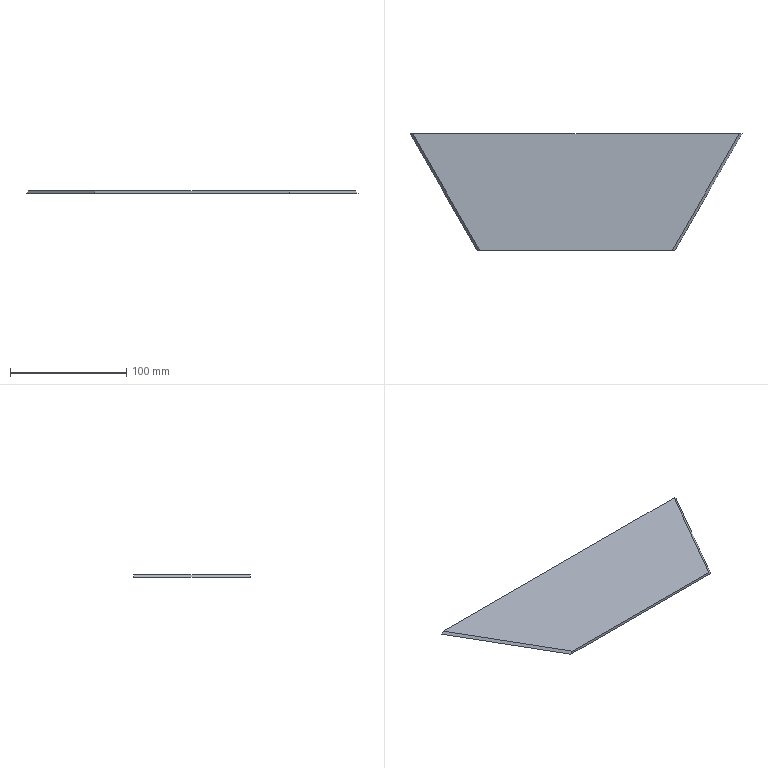Part | NX | 1 solid | 6 faces | box 285.47 x 100 x 2 mm | volume 45085 mm3 | plane 6
STEP:
#1=CARTESIAN_POINT('',(2.309,0.,2.));
#2=VERTEX_POINT('',#1);
#3=CARTESIAN_POINT('',(167.691,0.,2.));
#4=VERTEX_POINT('',#3);
#5=CARTESIAN_POINT('',(0.,0.,2.));
#6=DIRECTION('',(1.,0.,0.));
#7=VECTOR('',#6,1.);
#8=LINE('',#5,#7);
#9=EDGE_CURVE('',#2,#4,#8,.T.);
#10=ORIENTED_EDGE('',*,*,#9,.F.);
#11=CARTESIAN_POINT('',(0.,0.,0.));
#12=VERTEX_POINT('',#11);
#13=CARTESIAN_POINT('',(-31.012,0.,-26.857));
#14=DIRECTION('',(-0.7559,0.,-0.6547));
#15=VECTOR('',#14,1.);
#16=LINE('',#13,#15);
#17=EDGE_CURVE('',#2,#12,#16,.T.);
#18=ORIENTED_EDGE('',*,*,#17,.T.);
#19=CARTESIAN_POINT('',(170.,0.,0.));
#20=VERTEX_POINT('',#19);
#21=CARTESIAN_POINT('',(0.,0.,0.));
#22=DIRECTION('',(1.,0.,0.));
#23=VECTOR('',#22,1.);
#24=LINE('',#21,#23);
#25=EDGE_CURVE('',#12,#20,#24,.T.);
#26=ORIENTED_EDGE('',*,*,#25,.T.);
#27=CARTESIAN_POINT('',(160.231,0.,8.461));
#28=DIRECTION('',(-0.7559,0.,0.6547));
#29=VECTOR('',#28,1.);
#30=LINE('',#27,#29);
#31=EDGE_CURVE('',#20,#4,#30,.T.);
#32=ORIENTED_EDGE('',*,*,#31,.T.);
#33=EDGE_LOOP('',(#10,#18,#26,#32));
#34=FACE_OUTER_BOUND('',#33,.T.);
#35=CARTESIAN_POINT('',(0.,0.,2.));
#36=DIRECTION('',(0.,1.,0.));
#37=DIRECTION('',(0.,0.,1.));
#38=AXIS2_PLACEMENT_3D('',#35,#36,#37);
#39=PLANE('',#38);
#40=ADVANCED_FACE('',(#34),#39,.F.);
#41=CARTESIAN_POINT('',(227.735,100.,0.));
#42=VERTEX_POINT('',#41);
#43=CARTESIAN_POINT('',(-57.735,100.,0.));
#44=VERTEX_POINT('',#43);
#45=CARTESIAN_POINT('',(-57.735,100.,0.));
#46=DIRECTION('',(-1.,0.,0.));
#47=VECTOR('',#46,1.);
#48=LINE('',#45,#47);
#49=EDGE_CURVE('',#42,#44,#48,.T.);
#50=ORIENTED_EDGE('',*,*,#49,.T.);
#51=CARTESIAN_POINT('',(-55.426,100.,2.));
#52=VERTEX_POINT('',#51);
#53=CARTESIAN_POINT('',(-55.756,100.,1.714));
#54=DIRECTION('',(0.7559,0.,0.6547));
#55=VECTOR('',#54,1.);
#56=LINE('',#53,#55);
#57=EDGE_CURVE('',#44,#52,#56,.T.);
#58=ORIENTED_EDGE('',*,*,#57,.T.);
#59=CARTESIAN_POINT('',(225.426,100.,2.));
#60=VERTEX_POINT('',#59);
#61=CARTESIAN_POINT('',(-57.735,100.,2.));
#62=DIRECTION('',(-1.,0.,0.));
#63=VECTOR('',#62,1.);
#64=LINE('',#61,#63);
#65=EDGE_CURVE('',#60,#52,#64,.T.);
#66=ORIENTED_EDGE('',*,*,#65,.F.);
#67=CARTESIAN_POINT('',(184.974,100.,37.032));
#68=DIRECTION('',(0.7559,0.,-0.6547));
#69=VECTOR('',#68,1.);
#70=LINE('',#67,#69);
#71=EDGE_CURVE('',#60,#42,#70,.T.);
#72=ORIENTED_EDGE('',*,*,#71,.T.);
#73=EDGE_LOOP('',(#50,#58,#66,#72));
#74=FACE_OUTER_BOUND('',#73,.T.);
#75=CARTESIAN_POINT('',(-57.735,100.,2.));
#76=DIRECTION('',(0.,-1.,0.));
#77=DIRECTION('',(0.,0.,-1.));
#78=AXIS2_PLACEMENT_3D('',#75,#76,#77);
#79=PLANE('',#78);
#80=ADVANCED_FACE('',(#74),#79,.F.);
#81=ORIENTED_EDGE('',*,*,#65,.T.);
#82=CARTESIAN_POINT('',(-56.003,101.,2.));
#83=DIRECTION('',(0.5,-0.866,0.));
#84=VECTOR('',#83,1.);
#85=LINE('',#82,#84);
#86=EDGE_CURVE('',#52,#2,#85,.T.);
#87=ORIENTED_EDGE('',*,*,#86,.T.);
#88=ORIENTED_EDGE('',*,*,#9,.T.);
#89=CARTESIAN_POINT('',(154.635,-22.612,2.));
#90=DIRECTION('',(0.5,0.866,0.));
#91=VECTOR('',#90,1.);
#92=LINE('',#89,#91);
#93=EDGE_CURVE('',#4,#60,#92,.T.);
#94=ORIENTED_EDGE('',*,*,#93,.T.);
#95=EDGE_LOOP('',(#81,#87,#88,#94));
#96=FACE_OUTER_BOUND('',#95,.T.);
#97=CARTESIAN_POINT('',(-57.735,100.,2.));
#98=DIRECTION('',(0.,0.,-1.));
#99=DIRECTION('',(-1.,0.,0.));
#100=AXIS2_PLACEMENT_3D('',#97,#98,#99);
#101=PLANE('',#100);
#102=ADVANCED_FACE('',(#96),#101,.F.);
#103=CARTESIAN_POINT('',(0.,0.,0.));
#104=DIRECTION('',(0.5,-0.866,0.));
#105=VECTOR('',#104,1.);
#106=LINE('',#103,#105);
#107=EDGE_CURVE('',#44,#12,#106,.T.);
#108=ORIENTED_EDGE('',*,*,#107,.F.);
#109=ORIENTED_EDGE('',*,*,#49,.F.);
#110=CARTESIAN_POINT('',(170.,0.,0.));
#111=DIRECTION('',(0.5,0.866,0.));
#112=VECTOR('',#111,1.);
#113=LINE('',#110,#112);
#114=EDGE_CURVE('',#20,#42,#113,.T.);
#115=ORIENTED_EDGE('',*,*,#114,.F.);
#116=ORIENTED_EDGE('',*,*,#25,.F.);
#117=EDGE_LOOP('',(#108,#109,#115,#116));
#118=FACE_OUTER_BOUND('',#117,.T.);
#119=CARTESIAN_POINT('',(-57.735,100.,0.));
#120=DIRECTION('',(0.,0.,-1.));
#121=DIRECTION('',(-1.,0.,0.));
#122=AXIS2_PLACEMENT_3D('',#119,#120,#121);
#123=PLANE('',#122);
#124=ADVANCED_FACE('',(#118),#123,.T.);
#125=ORIENTED_EDGE('',*,*,#57,.F.);
#126=ORIENTED_EDGE('',*,*,#107,.T.);
#127=ORIENTED_EDGE('',*,*,#17,.F.);
#128=ORIENTED_EDGE('',*,*,#86,.F.);
#129=EDGE_LOOP('',(#125,#126,#127,#128));
#130=FACE_OUTER_BOUND('',#129,.T.);
#131=CARTESIAN_POINT('',(-56.003,101.,2.));
#132=DIRECTION('',(0.6124,0.3536,-0.7071));
#133=DIRECTION('',(-0.7559,0.,-0.6547));
#134=AXIS2_PLACEMENT_3D('',#131,#132,#133);
#135=PLANE('',#134);
#136=ADVANCED_FACE('',(#130),#135,.F.);
#137=ORIENTED_EDGE('',*,*,#31,.F.);
#138=ORIENTED_EDGE('',*,*,#114,.T.);
#139=ORIENTED_EDGE('',*,*,#71,.F.);
#140=ORIENTED_EDGE('',*,*,#93,.F.);
#141=EDGE_LOOP('',(#137,#138,#139,#140));
#142=FACE_OUTER_BOUND('',#141,.T.);
#143=CARTESIAN_POINT('',(154.635,-22.612,2.));
#144=DIRECTION('',(-0.6124,0.3536,-0.7071));
#145=DIRECTION('',(-0.7559,0.,0.6547));
#146=AXIS2_PLACEMENT_3D('',#143,#144,#145);
#147=PLANE('',#146);
#148=ADVANCED_FACE('',(#142),#147,.F.);
#149=CLOSED_SHELL('',(#40,#80,#102,#124,#136,#148));
#150=MANIFOLD_SOLID_BREP('',#149);
#151=(LENGTH_UNIT()NAMED_UNIT(*)SI_UNIT(.MILLI.,.METRE.));
#152=UNCERTAINTY_MEASURE_WITH_UNIT(LENGTH_MEASURE(0.00002),#151,'','');
#153=(NAMED_UNIT(*)PLANE_ANGLE_UNIT()SI_UNIT($,.RADIAN.));
#154=PLANE_ANGLE_MEASURE_WITH_UNIT(PLANE_ANGLE_MEASURE(0.01745),#153);
#155=DIMENSIONAL_EXPONENTS(0.,0.,0.,0.,0.,0.,0.);
#156=(CONVERSION_BASED_UNIT('DEGREE',#154)NAMED_UNIT(#155)PLANE_ANGLE_UNIT());
#157=(NAMED_UNIT(*)SI_UNIT($,.STERADIAN.)SOLID_ANGLE_UNIT());
#158=(GEOMETRIC_REPRESENTATION_CONTEXT(3)GLOBAL_UNCERTAINTY_ASSIGNED_CONTEXT((#152))GLOBAL_UNIT_ASSIGNED_CONTEXT((#151,#156,#157))REPRESENTATION_CONTEXT('',''));
#159=ADVANCED_BREP_SHAPE_REPRESENTATION('',(#150),#158);